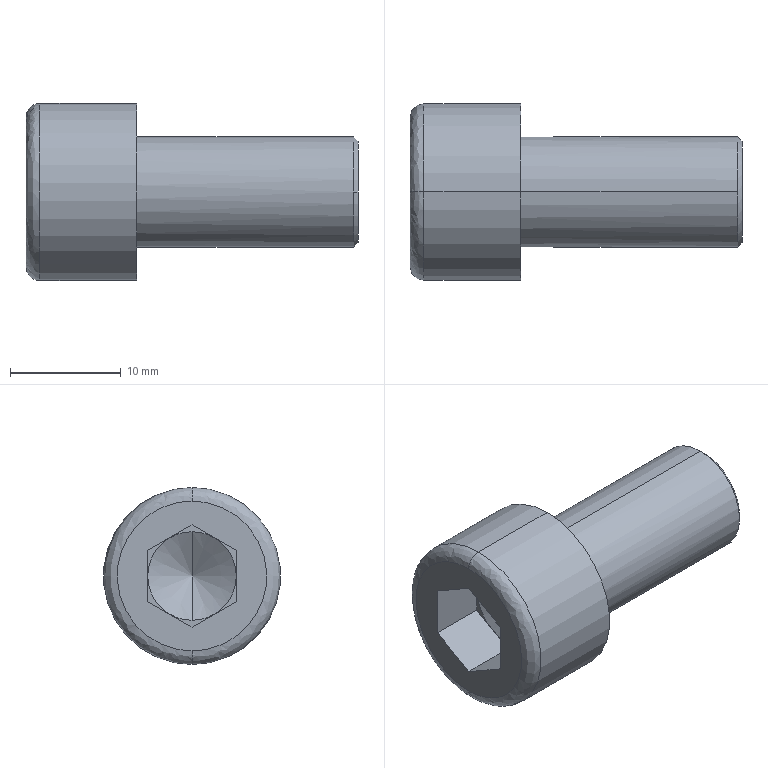Part | STEP file | hexagon socket head cap screws_gb_GB_FASTENER_SCREWS_HSHCS M10X20-N | 1 solid | 25 faces | box 30 x 16 x 16 mm | volume 3247 mm3 | plane 15 | cylinder 4 | cone 4 | spline 2 | commonest cylinder face diameters 10 x2 16 x2